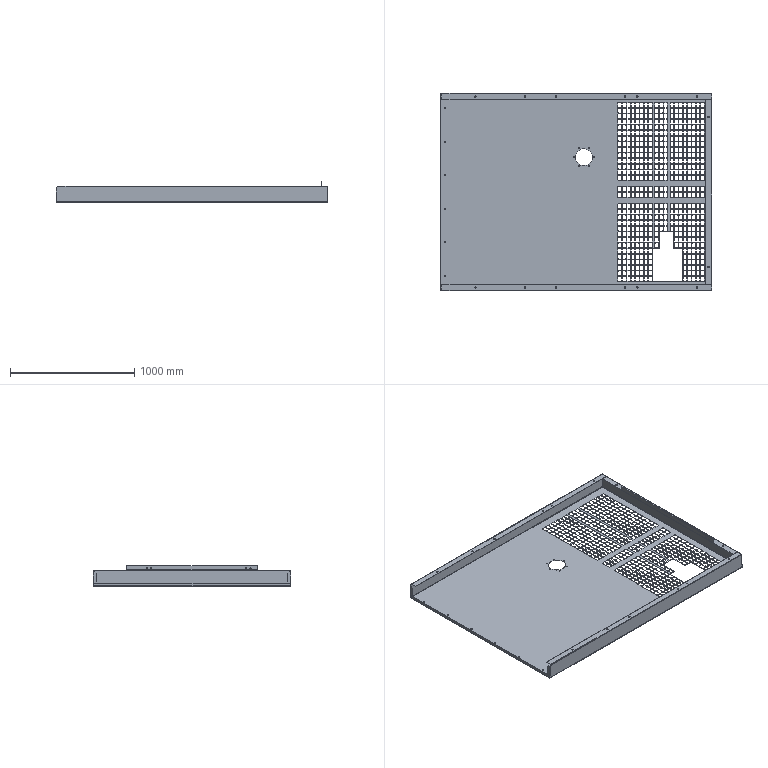Part | STEP file | SYL_0392D6J1SYL0380DJ100-163725 | 1 solid | 4420 faces | volume 7732310 mm3 | plane 2210 | cylinder 2202 | spline 8 | commonest cylinder face diameters 5 x2100 10.5 x40 8 x22 10 x16 11 x12 4 x10